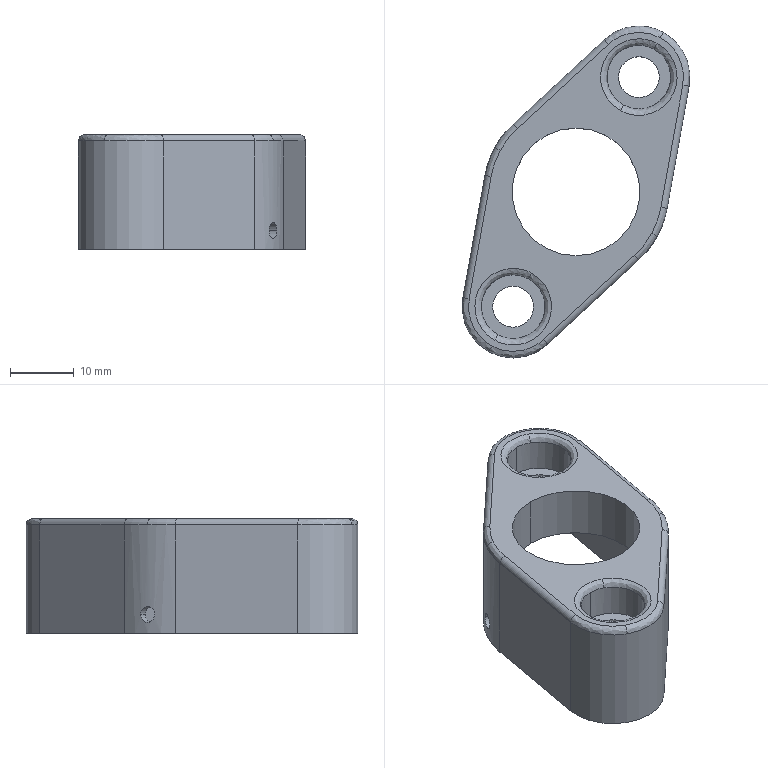Part | SolidWorks | features BaseBody 1 | 1 solid | 53 faces | box 35.676 x 51.97 x 18 mm | volume 7698 mm3 | cylinder 28 | plane 13 | spline 12 | commonest cylinder face diameters 2 x4 2.5 x4 6.4 x4 10 x4 13 x3 16 x3